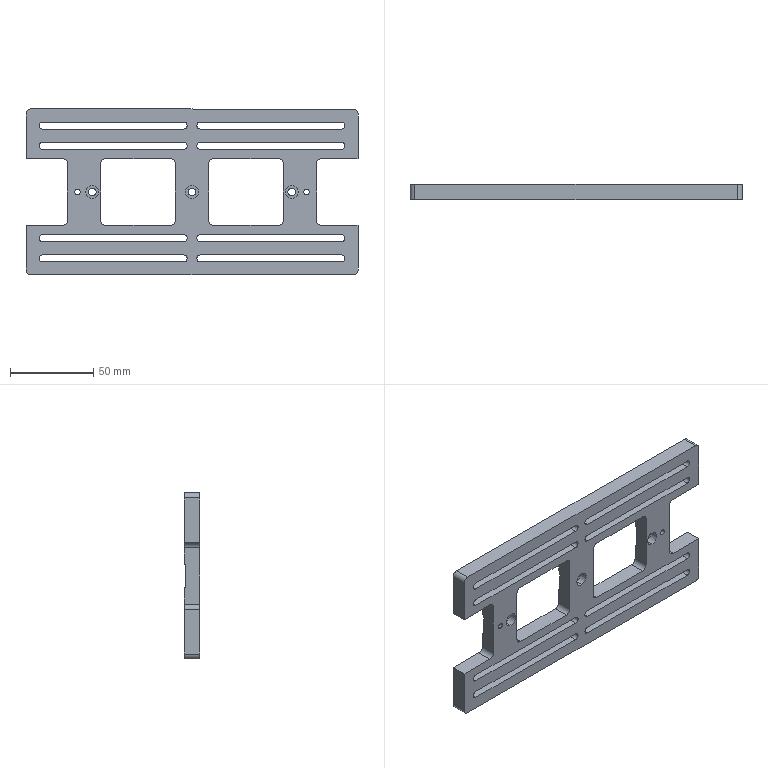Part | SolidWorks | features ICE 5, Fillet 3, MirrorPattern 3, HoleWzd 2, Extrusion 1 | 1 solid | 139 faces | box 200 x 9.4 x 100 mm | volume 91382 mm3 | plane 75 | cylinder 64 | commonest cylinder face diameters 8 x22 4.2 x16 6 x16 4.5 x6 3.3 x4